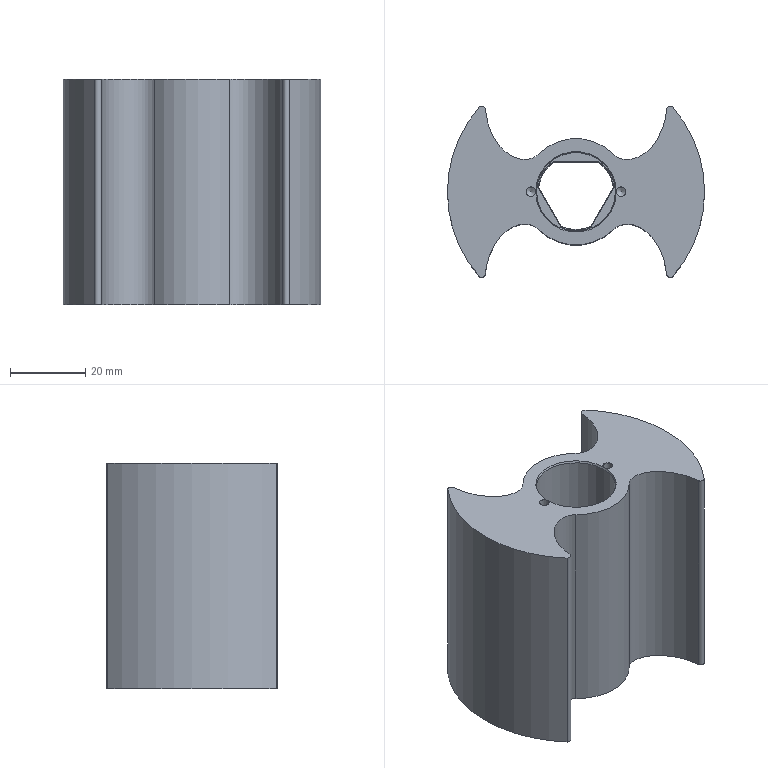NC program | NX | posted with a generic post | part box 68.489 x 45.577 x 60 mm
Lines 6961 to 7016 of 7016:
(PLANAR_MILL_COPY_COPY , TOOL : D6A45)
N13914 T07 M6
N13916 G54
N13918 G17 G0 G90 X-14.057 Y-9.915 S7500 M3
N13920 G43 Z30. H7
N13922 Z1.5
N13924 G94 G1 Z-1.5 F1250.
N13926 G3 X-14.883 Y-9.734 R1.
N13928 X-15.536 Y-9.917 R6.491
N13930 X-17.945 Y-11.232 R7.917
N13932 X-19.961 Y-13.282 R11.975
N13934 X-22.165 Y-17.373 R14.386
N13936 X-23.192 Y-22.033 R20.75
N13938 G2 X-26.604 Y-23.118 R1.95
N13940 X-26.604 Y23.118 R35.245
N13942 X-23.192 Y22.033 R1.95
N13944 G3 X-22.164 Y17.371 R20.747
N13946 X-19.958 Y13.279 R14.385
N13948 X-17.799 Y11.118 R11.932
N13950 X-15.21 Y9.816 R7.617
N13952 X-13.967 Y9.6 R6.192
N13954 X-12.762 Y9.668 R4.761
N13956 X-11.645 Y10.046 R4.149
N13958 X-10.715 Y10.717 R3.674
N13960 G2 X10.715 Y10.717 R15.155
N13962 G3 X11.713 Y10.012 R3.672
N13964 X12.92 Y9.642 R4.229
N13966 X14.214 Y9.621 R4.908
N13968 X15.536 Y9.917 R6.491
N13970 X17.945 Y11.232 R7.917
N13972 X19.961 Y13.282 R11.975
N13974 X22.165 Y17.373 R14.386
N13976 X23.192 Y22.033 R20.75
N13978 G2 X26.604 Y23.118 R1.95
N13980 X26.604 Y-23.118 R35.245
N13982 X23.192 Y-22.033 R1.95
N13984 G3 X22.164 Y-17.371 R20.747
N13986 X19.958 Y-13.279 R14.385
N13988 X17.799 Y-11.118 R11.932
N13990 X15.21 Y-9.816 R7.617
N13992 X13.967 Y-9.6 R6.192
N13994 X12.762 Y-9.668 R4.761
N13996 X11.645 Y-10.046 R4.149
N13998 X10.715 Y-10.717 R3.674
N14000 G2 X-10.715 Y-10.717 R15.155
N14002 G3 X-11.713 Y-10.012 R3.672
N14004 X-12.92 Y-9.642 R4.229
N14006 X-14.214 Y-9.621 R4.908
N14008 X-14.883 Y-9.734 R6.491
N14010 X-15.552 Y-10.251 R1.
N14012 G1 Z1.5
N14014 G0 Z30.
N14016 M5
N14018 M2